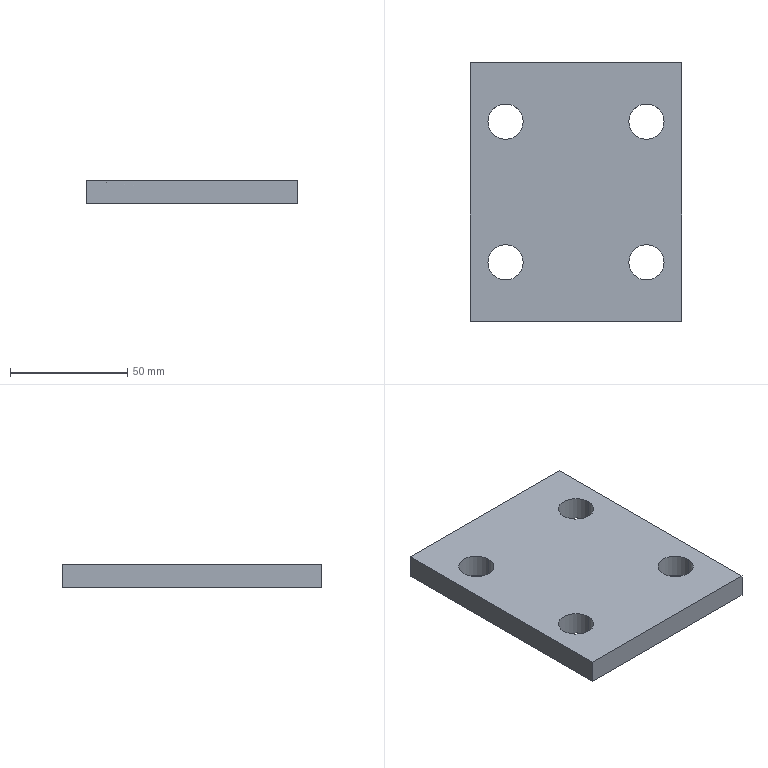Part | SolidWorks | features ICE 2, Extrusion 1 | 1 solid | 14 faces | box 90 x 110 x 10 mm | volume 91931 mm3 | cylinder 8 | plane 6 | commonest cylinder face diameters 15 x8
STEP:
#1=CARTESIAN_POINT('',(72.5,30.,0.));
#2=VERTEX_POINT('',#1);
#3=CARTESIAN_POINT('',(87.5,30.,0.));
#4=VERTEX_POINT('',#3);
#5=CARTESIAN_POINT('',(80.,30.,0.));
#6=DIRECTION('',(0.,0.,1.));
#7=DIRECTION('',(1.,0.,0.));
#8=AXIS2_PLACEMENT_3D('',#5,#6,#7);
#9=CIRCLE('',#8,7.5);
#10=EDGE_CURVE('',#2,#4,#9,.T.);
#11=ORIENTED_EDGE('',*,*,#10,.F.);
#12=CARTESIAN_POINT('',(72.5,30.,10.));
#13=VERTEX_POINT('',#12);
#14=CARTESIAN_POINT('',(72.5,30.,0.));
#15=DIRECTION('',(0.,0.,1.));
#16=VECTOR('',#15,1000.);
#17=LINE('',#14,#16);
#18=EDGE_CURVE('',#2,#13,#17,.T.);
#19=ORIENTED_EDGE('',*,*,#18,.T.);
#20=CARTESIAN_POINT('',(87.5,30.,10.));
#21=VERTEX_POINT('',#20);
#22=CARTESIAN_POINT('',(80.,30.,10.));
#23=DIRECTION('',(0.,0.,1.));
#24=DIRECTION('',(1.,0.,0.));
#25=AXIS2_PLACEMENT_3D('',#22,#23,#24);
#26=CIRCLE('',#25,7.5);
#27=EDGE_CURVE('',#13,#21,#26,.T.);
#28=ORIENTED_EDGE('',*,*,#27,.T.);
#29=CARTESIAN_POINT('',(87.5,30.,0.));
#30=DIRECTION('',(0.,0.,1.));
#31=VECTOR('',#30,1000.);
#32=LINE('',#29,#31);
#33=EDGE_CURVE('',#4,#21,#32,.T.);
#34=ORIENTED_EDGE('',*,*,#33,.F.);
#35=EDGE_LOOP('',(#11,#19,#28,#34));
#36=FACE_OUTER_BOUND('',#35,.T.);
#37=CARTESIAN_POINT('',(80.,30.,0.));
#38=DIRECTION('',(0.,0.,1.));
#39=DIRECTION('',(1.,0.,0.));
#40=AXIS2_PLACEMENT_3D('',#37,#38,#39);
#41=CYLINDRICAL_SURFACE('',#40,7.5);
#42=ADVANCED_FACE('',(#36),#41,.F.);
#43=CARTESIAN_POINT('',(12.5,30.,0.));
#44=VERTEX_POINT('',#43);
#45=CARTESIAN_POINT('',(27.5,30.,0.));
#46=VERTEX_POINT('',#45);
#47=CARTESIAN_POINT('',(20.,30.,0.));
#48=DIRECTION('',(0.,0.,1.));
#49=DIRECTION('',(1.,0.,0.));
#50=AXIS2_PLACEMENT_3D('',#47,#48,#49);
#51=CIRCLE('',#50,7.5);
#52=EDGE_CURVE('',#44,#46,#51,.T.);
#53=ORIENTED_EDGE('',*,*,#52,.F.);
#54=CARTESIAN_POINT('',(12.5,30.,10.));
#55=VERTEX_POINT('',#54);
#56=CARTESIAN_POINT('',(12.5,30.,0.));
#57=DIRECTION('',(0.,0.,1.));
#58=VECTOR('',#57,1000.);
#59=LINE('',#56,#58);
#60=EDGE_CURVE('',#44,#55,#59,.T.);
#61=ORIENTED_EDGE('',*,*,#60,.T.);
#62=CARTESIAN_POINT('',(27.5,30.,10.));
#63=VERTEX_POINT('',#62);
#64=CARTESIAN_POINT('',(20.,30.,10.));
#65=DIRECTION('',(0.,0.,1.));
#66=DIRECTION('',(1.,0.,0.));
#67=AXIS2_PLACEMENT_3D('',#64,#65,#66);
#68=CIRCLE('',#67,7.5);
#69=EDGE_CURVE('',#55,#63,#68,.T.);
#70=ORIENTED_EDGE('',*,*,#69,.T.);
#71=CARTESIAN_POINT('',(27.5,30.,0.));
#72=DIRECTION('',(0.,0.,1.));
#73=VECTOR('',#72,1000.);
#74=LINE('',#71,#73);
#75=EDGE_CURVE('',#46,#63,#74,.T.);
#76=ORIENTED_EDGE('',*,*,#75,.F.);
#77=EDGE_LOOP('',(#53,#61,#70,#76));
#78=FACE_OUTER_BOUND('',#77,.T.);
#79=CARTESIAN_POINT('',(20.,30.,0.));
#80=DIRECTION('',(0.,0.,1.));
#81=DIRECTION('',(1.,0.,0.));
#82=AXIS2_PLACEMENT_3D('',#79,#80,#81);
#83=CYLINDRICAL_SURFACE('',#82,7.5);
#84=ADVANCED_FACE('',(#78),#83,.F.);
#85=CARTESIAN_POINT('',(12.5,90.,0.));
#86=VERTEX_POINT('',#85);
#87=CARTESIAN_POINT('',(27.5,90.,0.));
#88=VERTEX_POINT('',#87);
#89=CARTESIAN_POINT('',(20.,90.,0.));
#90=DIRECTION('',(0.,0.,1.));
#91=DIRECTION('',(1.,0.,0.));
#92=AXIS2_PLACEMENT_3D('',#89,#90,#91);
#93=CIRCLE('',#92,7.5);
#94=EDGE_CURVE('',#86,#88,#93,.T.);
#95=ORIENTED_EDGE('',*,*,#94,.F.);
#96=CARTESIAN_POINT('',(12.5,90.,10.));
#97=VERTEX_POINT('',#96);
#98=CARTESIAN_POINT('',(12.5,90.,0.));
#99=DIRECTION('',(0.,0.,1.));
#100=VECTOR('',#99,1000.);
#101=LINE('',#98,#100);
#102=EDGE_CURVE('',#86,#97,#101,.T.);
#103=ORIENTED_EDGE('',*,*,#102,.T.);
#104=CARTESIAN_POINT('',(27.5,90.,10.));
#105=VERTEX_POINT('',#104);
#106=CARTESIAN_POINT('',(20.,90.,10.));
#107=DIRECTION('',(0.,0.,1.));
#108=DIRECTION('',(1.,0.,0.));
#109=AXIS2_PLACEMENT_3D('',#106,#107,#108);
#110=CIRCLE('',#109,7.5);
#111=EDGE_CURVE('',#97,#105,#110,.T.);
#112=ORIENTED_EDGE('',*,*,#111,.T.);
#113=CARTESIAN_POINT('',(27.5,90.,0.));
#114=DIRECTION('',(0.,0.,1.));
#115=VECTOR('',#114,1000.);
#116=LINE('',#113,#115);
#117=EDGE_CURVE('',#88,#105,#116,.T.);
#118=ORIENTED_EDGE('',*,*,#117,.F.);
#119=EDGE_LOOP('',(#95,#103,#112,#118));
#120=FACE_OUTER_BOUND('',#119,.T.);
#121=CARTESIAN_POINT('',(20.,90.,0.));
#122=DIRECTION('',(0.,0.,1.));
#123=DIRECTION('',(1.,0.,0.));
#124=AXIS2_PLACEMENT_3D('',#121,#122,#123);
#125=CYLINDRICAL_SURFACE('',#124,7.5);
#126=ADVANCED_FACE('',(#120),#125,.F.);
#127=CARTESIAN_POINT('',(72.5,90.,0.));
#128=VERTEX_POINT('',#127);
#129=CARTESIAN_POINT('',(87.5,90.,0.));
#130=VERTEX_POINT('',#129);
#131=CARTESIAN_POINT('',(80.,90.,0.));
#132=DIRECTION('',(0.,0.,1.));
#133=DIRECTION('',(1.,0.,0.));
#134=AXIS2_PLACEMENT_3D('',#131,#132,#133);
#135=CIRCLE('',#134,7.5);
#136=EDGE_CURVE('',#128,#130,#135,.T.);
#137=ORIENTED_EDGE('',*,*,#136,.F.);
#138=CARTESIAN_POINT('',(72.5,90.,10.));
#139=VERTEX_POINT('',#138);
#140=CARTESIAN_POINT('',(72.5,90.,0.));
#141=DIRECTION('',(0.,0.,1.));
#142=VECTOR('',#141,1000.);
#143=LINE('',#140,#142);
#144=EDGE_CURVE('',#128,#139,#143,.T.);
#145=ORIENTED_EDGE('',*,*,#144,.T.);
#146=CARTESIAN_POINT('',(87.5,90.,10.));
#147=VERTEX_POINT('',#146);
#148=CARTESIAN_POINT('',(80.,90.,10.));
#149=DIRECTION('',(0.,0.,1.));
#150=DIRECTION('',(1.,0.,0.));
#151=AXIS2_PLACEMENT_3D('',#148,#149,#150);
#152=CIRCLE('',#151,7.5);
#153=EDGE_CURVE('',#139,#147,#152,.T.);
#154=ORIENTED_EDGE('',*,*,#153,.T.);
#155=CARTESIAN_POINT('',(87.5,90.,0.));
#156=DIRECTION('',(0.,0.,1.));
#157=VECTOR('',#156,1000.);
#158=LINE('',#155,#157);
#159=EDGE_CURVE('',#130,#147,#158,.T.);
#160=ORIENTED_EDGE('',*,*,#159,.F.);
#161=EDGE_LOOP('',(#137,#145,#154,#160));
#162=FACE_OUTER_BOUND('',#161,.T.);
#163=CARTESIAN_POINT('',(80.,90.,0.));
#164=DIRECTION('',(0.,0.,1.));
#165=DIRECTION('',(1.,0.,0.));
#166=AXIS2_PLACEMENT_3D('',#163,#164,#165);
#167=CYLINDRICAL_SURFACE('',#166,7.5);
#168=ADVANCED_FACE('',(#162),#167,.F.);
#169=CARTESIAN_POINT('',(80.,90.,10.));
#170=DIRECTION('',(0.,0.,1.));
#171=DIRECTION('',(1.,0.,0.));
#172=AXIS2_PLACEMENT_3D('',#169,#170,#171);
#173=CIRCLE('',#172,7.5);
#174=EDGE_CURVE('',#147,#139,#173,.T.);
#175=ORIENTED_EDGE('',*,*,#174,.F.);
#176=ORIENTED_EDGE('',*,*,#153,.F.);
#177=EDGE_LOOP('',(#175,#176));
#178=FACE_BOUND('',#177,.T.);
#179=CARTESIAN_POINT('',(20.,90.,10.));
#180=DIRECTION('',(0.,0.,1.));
#181=DIRECTION('',(1.,0.,0.));
#182=AXIS2_PLACEMENT_3D('',#179,#180,#181);
#183=CIRCLE('',#182,7.5);
#184=EDGE_CURVE('',#105,#97,#183,.T.);
#185=ORIENTED_EDGE('',*,*,#184,.F.);
#186=ORIENTED_EDGE('',*,*,#111,.F.);
#187=EDGE_LOOP('',(#185,#186));
#188=FACE_BOUND('',#187,.T.);
#189=CARTESIAN_POINT('',(20.,30.,10.));
#190=DIRECTION('',(0.,0.,1.));
#191=DIRECTION('',(1.,0.,0.));
#192=AXIS2_PLACEMENT_3D('',#189,#190,#191);
#193=CIRCLE('',#192,7.5);
#194=EDGE_CURVE('',#63,#55,#193,.T.);
#195=ORIENTED_EDGE('',*,*,#194,.F.);
#196=ORIENTED_EDGE('',*,*,#69,.F.);
#197=EDGE_LOOP('',(#195,#196));
#198=FACE_BOUND('',#197,.T.);
#199=CARTESIAN_POINT('',(80.,30.,10.));
#200=DIRECTION('',(0.,0.,1.));
#201=DIRECTION('',(1.,0.,0.));
#202=AXIS2_PLACEMENT_3D('',#199,#200,#201);
#203=CIRCLE('',#202,7.5);
#204=EDGE_CURVE('',#21,#13,#203,.T.);
#205=ORIENTED_EDGE('',*,*,#204,.F.);
#206=ORIENTED_EDGE('',*,*,#27,.F.);
#207=EDGE_LOOP('',(#205,#206));
#208=FACE_BOUND('',#207,.T.);
#209=CARTESIAN_POINT('',(95.,5.,10.));
#210=VERTEX_POINT('',#209);
#211=CARTESIAN_POINT('',(95.,115.,10.));
#212=VERTEX_POINT('',#211);
#213=CARTESIAN_POINT('',(95.,60.,10.));
#214=DIRECTION('',(0.,1.,0.));
#215=VECTOR('',#214,1000.);
#216=LINE('',#213,#215);
#217=EDGE_CURVE('',#210,#212,#216,.T.);
#218=ORIENTED_EDGE('',*,*,#217,.T.);
#219=CARTESIAN_POINT('',(5.,115.,10.));
#220=VERTEX_POINT('',#219);
#221=CARTESIAN_POINT('',(95.,115.,10.));
#222=DIRECTION('',(-1.,0.,0.));
#223=VECTOR('',#222,1000.);
#224=LINE('',#221,#223);
#225=EDGE_CURVE('',#212,#220,#224,.T.);
#226=ORIENTED_EDGE('',*,*,#225,.T.);
#227=CARTESIAN_POINT('',(5.,5.,10.));
#228=VERTEX_POINT('',#227);
#229=CARTESIAN_POINT('',(5.,115.,10.));
#230=DIRECTION('',(0.,-1.,0.));
#231=VECTOR('',#230,1000.);
#232=LINE('',#229,#231);
#233=EDGE_CURVE('',#220,#228,#232,.T.);
#234=ORIENTED_EDGE('',*,*,#233,.T.);
#235=CARTESIAN_POINT('',(5.,5.,10.));
#236=DIRECTION('',(1.,0.,0.));
#237=VECTOR('',#236,1000.);
#238=LINE('',#235,#237);
#239=EDGE_CURVE('',#228,#210,#238,.T.);
#240=ORIENTED_EDGE('',*,*,#239,.T.);
#241=EDGE_LOOP('',(#218,#226,#234,#240));
#242=FACE_OUTER_BOUND('',#241,.T.);
#243=CARTESIAN_POINT('',(0.,0.,10.));
#244=DIRECTION('',(0.,0.,-1.));
#245=DIRECTION('',(-1.,0.,0.));
#246=AXIS2_PLACEMENT_3D('',#243,#244,#245);
#247=PLANE('',#246);
#248=ADVANCED_FACE('',(#178,#188,#198,#208,#242),#247,.F.);
#249=CARTESIAN_POINT('',(80.,90.,0.));
#250=DIRECTION('',(0.,0.,1.));
#251=DIRECTION('',(1.,0.,0.));
#252=AXIS2_PLACEMENT_3D('',#249,#250,#251);
#253=CIRCLE('',#252,7.5);
#254=EDGE_CURVE('',#130,#128,#253,.T.);
#255=ORIENTED_EDGE('',*,*,#254,.T.);
#256=ORIENTED_EDGE('',*,*,#136,.T.);
#257=EDGE_LOOP('',(#255,#256));
#258=FACE_BOUND('',#257,.T.);
#259=CARTESIAN_POINT('',(20.,90.,0.));
#260=DIRECTION('',(0.,0.,1.));
#261=DIRECTION('',(1.,0.,0.));
#262=AXIS2_PLACEMENT_3D('',#259,#260,#261);
#263=CIRCLE('',#262,7.5);
#264=EDGE_CURVE('',#88,#86,#263,.T.);
#265=ORIENTED_EDGE('',*,*,#264,.T.);
#266=ORIENTED_EDGE('',*,*,#94,.T.);
#267=EDGE_LOOP('',(#265,#266));
#268=FACE_BOUND('',#267,.T.);
#269=CARTESIAN_POINT('',(20.,30.,0.));
#270=DIRECTION('',(0.,0.,1.));
#271=DIRECTION('',(1.,0.,0.));
#272=AXIS2_PLACEMENT_3D('',#269,#270,#271);
#273=CIRCLE('',#272,7.5);
#274=EDGE_CURVE('',#46,#44,#273,.T.);
#275=ORIENTED_EDGE('',*,*,#274,.T.);
#276=ORIENTED_EDGE('',*,*,#52,.T.);
#277=EDGE_LOOP('',(#275,#276));
#278=FACE_BOUND('',#277,.T.);
#279=CARTESIAN_POINT('',(80.,30.,0.));
#280=DIRECTION('',(0.,0.,1.));
#281=DIRECTION('',(1.,0.,0.));
#282=AXIS2_PLACEMENT_3D('',#279,#280,#281);
#283=CIRCLE('',#282,7.5);
#284=EDGE_CURVE('',#4,#2,#283,.T.);
#285=ORIENTED_EDGE('',*,*,#284,.T.);
#286=ORIENTED_EDGE('',*,*,#10,.T.);
#287=EDGE_LOOP('',(#285,#286));
#288=FACE_BOUND('',#287,.T.);
#289=CARTESIAN_POINT('',(95.,115.,0.));
#290=VERTEX_POINT('',#289);
#291=CARTESIAN_POINT('',(5.,115.,0.));
#292=VERTEX_POINT('',#291);
#293=CARTESIAN_POINT('',(95.,115.,0.));
#294=DIRECTION('',(-1.,0.,0.));
#295=VECTOR('',#294,1000.);
#296=LINE('',#293,#295);
#297=EDGE_CURVE('',#290,#292,#296,.T.);
#298=ORIENTED_EDGE('',*,*,#297,.F.);
#299=CARTESIAN_POINT('',(95.,5.,0.));
#300=VERTEX_POINT('',#299);
#301=CARTESIAN_POINT('',(95.,60.,0.));
#302=DIRECTION('',(0.,1.,0.));
#303=VECTOR('',#302,1000.);
#304=LINE('',#301,#303);
#305=EDGE_CURVE('',#300,#290,#304,.T.);
#306=ORIENTED_EDGE('',*,*,#305,.F.);
#307=CARTESIAN_POINT('',(5.,5.,0.));
#308=VERTEX_POINT('',#307);
#309=CARTESIAN_POINT('',(5.,5.,0.));
#310=DIRECTION('',(1.,0.,0.));
#311=VECTOR('',#310,1000.);
#312=LINE('',#309,#311);
#313=EDGE_CURVE('',#308,#300,#312,.T.);
#314=ORIENTED_EDGE('',*,*,#313,.F.);
#315=CARTESIAN_POINT('',(5.,115.,0.));
#316=DIRECTION('',(0.,-1.,0.));
#317=VECTOR('',#316,1000.);
#318=LINE('',#315,#317);
#319=EDGE_CURVE('',#292,#308,#318,.T.);
#320=ORIENTED_EDGE('',*,*,#319,.F.);
#321=EDGE_LOOP('',(#298,#306,#314,#320));
#322=FACE_OUTER_BOUND('',#321,.T.);
#323=CARTESIAN_POINT('',(0.,0.,0.));
#324=DIRECTION('',(0.,0.,-1.));
#325=DIRECTION('',(-1.,0.,0.));
#326=AXIS2_PLACEMENT_3D('',#323,#324,#325);
#327=PLANE('',#326);
#328=ADVANCED_FACE('',(#258,#268,#278,#288,#322),#327,.T.);
#329=ORIENTED_EDGE('',*,*,#144,.F.);
#330=ORIENTED_EDGE('',*,*,#254,.F.);
#331=ORIENTED_EDGE('',*,*,#159,.T.);
#332=ORIENTED_EDGE('',*,*,#174,.T.);
#333=EDGE_LOOP('',(#329,#330,#331,#332));
#334=FACE_OUTER_BOUND('',#333,.T.);
#335=CARTESIAN_POINT('',(80.,90.,0.));
#336=DIRECTION('',(0.,0.,1.));
#337=DIRECTION('',(1.,0.,0.));
#338=AXIS2_PLACEMENT_3D('',#335,#336,#337);
#339=CYLINDRICAL_SURFACE('',#338,7.5);
#340=ADVANCED_FACE('',(#334),#339,.F.);
#341=ORIENTED_EDGE('',*,*,#102,.F.);
#342=ORIENTED_EDGE('',*,*,#264,.F.);
#343=ORIENTED_EDGE('',*,*,#117,.T.);
#344=ORIENTED_EDGE('',*,*,#184,.T.);
#345=EDGE_LOOP('',(#341,#342,#343,#344));
#346=FACE_OUTER_BOUND('',#345,.T.);
#347=CARTESIAN_POINT('',(20.,90.,0.));
#348=DIRECTION('',(0.,0.,1.));
#349=DIRECTION('',(1.,0.,0.));
#350=AXIS2_PLACEMENT_3D('',#347,#348,#349);
#351=CYLINDRICAL_SURFACE('',#350,7.5);
#352=ADVANCED_FACE('',(#346),#351,.F.);
#353=ORIENTED_EDGE('',*,*,#60,.F.);
#354=ORIENTED_EDGE('',*,*,#274,.F.);
#355=ORIENTED_EDGE('',*,*,#75,.T.);
#356=ORIENTED_EDGE('',*,*,#194,.T.);
#357=EDGE_LOOP('',(#353,#354,#355,#356));
#358=FACE_OUTER_BOUND('',#357,.T.);
#359=CARTESIAN_POINT('',(20.,30.,0.));
#360=DIRECTION('',(0.,0.,1.));
#361=DIRECTION('',(1.,0.,0.));
#362=AXIS2_PLACEMENT_3D('',#359,#360,#361);
#363=CYLINDRICAL_SURFACE('',#362,7.5);
#364=ADVANCED_FACE('',(#358),#363,.F.);
#365=ORIENTED_EDGE('',*,*,#18,.F.);
#366=ORIENTED_EDGE('',*,*,#284,.F.);
#367=ORIENTED_EDGE('',*,*,#33,.T.);
#368=ORIENTED_EDGE('',*,*,#204,.T.);
#369=EDGE_LOOP('',(#365,#366,#367,#368));
#370=FACE_OUTER_BOUND('',#369,.T.);
#371=CARTESIAN_POINT('',(80.,30.,0.));
#372=DIRECTION('',(0.,0.,1.));
#373=DIRECTION('',(1.,0.,0.));
#374=AXIS2_PLACEMENT_3D('',#371,#372,#373);
#375=CYLINDRICAL_SURFACE('',#374,7.5);
#376=ADVANCED_FACE('',(#370),#375,.F.);
#377=ORIENTED_EDGE('',*,*,#217,.F.);
#378=CARTESIAN_POINT('',(95.,5.,0.));
#379=DIRECTION('',(0.,0.,1.));
#380=VECTOR('',#379,1000.);
#381=LINE('',#378,#380);
#382=EDGE_CURVE('',#300,#210,#381,.T.);
#383=ORIENTED_EDGE('',*,*,#382,.F.);
#384=ORIENTED_EDGE('',*,*,#305,.T.);
#385=CARTESIAN_POINT('',(95.,115.,0.));
#386=DIRECTION('',(0.,0.,1.));
#387=VECTOR('',#386,1000.);
#388=LINE('',#385,#387);
#389=EDGE_CURVE('',#290,#212,#388,.T.);
#390=ORIENTED_EDGE('',*,*,#389,.T.);
#391=EDGE_LOOP('',(#377,#383,#384,#390));
#392=FACE_OUTER_BOUND('',#391,.T.);
#393=CARTESIAN_POINT('',(95.,60.,0.));
#394=DIRECTION('',(1.,0.,0.));
#395=DIRECTION('',(0.,0.,-1.));
#396=AXIS2_PLACEMENT_3D('',#393,#394,#395);
#397=PLANE('',#396);
#398=ADVANCED_FACE('',(#392),#397,.T.);
#399=ORIENTED_EDGE('',*,*,#239,.F.);
#400=CARTESIAN_POINT('',(5.,5.,0.));
#401=DIRECTION('',(0.,0.,1.));
#402=VECTOR('',#401,1000.);
#403=LINE('',#400,#402);
#404=EDGE_CURVE('',#308,#228,#403,.T.);
#405=ORIENTED_EDGE('',*,*,#404,.F.);
#406=ORIENTED_EDGE('',*,*,#313,.T.);
#407=ORIENTED_EDGE('',*,*,#382,.T.);
#408=EDGE_LOOP('',(#399,#405,#406,#407));
#409=FACE_OUTER_BOUND('',#408,.T.);
#410=CARTESIAN_POINT('',(5.,5.,0.));
#411=DIRECTION('',(0.,-1.,0.));
#412=DIRECTION('',(0.,0.,-1.));
#413=AXIS2_PLACEMENT_3D('',#410,#411,#412);
#414=PLANE('',#413);
#415=ADVANCED_FACE('',(#409),#414,.T.);
#416=ORIENTED_EDGE('',*,*,#233,.F.);
#417=CARTESIAN_POINT('',(5.,115.,0.));
#418=DIRECTION('',(0.,0.,1.));
#419=VECTOR('',#418,1000.);
#420=LINE('',#417,#419);
#421=EDGE_CURVE('',#292,#220,#420,.T.);
#422=ORIENTED_EDGE('',*,*,#421,.F.);
#423=ORIENTED_EDGE('',*,*,#319,.T.);
#424=ORIENTED_EDGE('',*,*,#404,.T.);
#425=EDGE_LOOP('',(#416,#422,#423,#424));
#426=FACE_OUTER_BOUND('',#425,.T.);
#427=CARTESIAN_POINT('',(5.,115.,0.));
#428=DIRECTION('',(-1.,0.,0.));
#429=DIRECTION('',(0.,0.,1.));
#430=AXIS2_PLACEMENT_3D('',#427,#428,#429);
#431=PLANE('',#430);
#432=ADVANCED_FACE('',(#426),#431,.T.);
#433=ORIENTED_EDGE('',*,*,#225,.F.);
#434=ORIENTED_EDGE('',*,*,#389,.F.);
#435=ORIENTED_EDGE('',*,*,#297,.T.);
#436=ORIENTED_EDGE('',*,*,#421,.T.);
#437=EDGE_LOOP('',(#433,#434,#435,#436));
#438=FACE_OUTER_BOUND('',#437,.T.);
#439=CARTESIAN_POINT('',(95.,115.,0.));
#440=DIRECTION('',(0.,1.,0.));
#441=DIRECTION('',(0.,0.,1.));
#442=AXIS2_PLACEMENT_3D('',#439,#440,#441);
#443=PLANE('',#442);
#444=ADVANCED_FACE('',(#438),#443,.T.);
#445=CLOSED_SHELL('',(#42,#84,#126,#168,#248,#328,#340,#352,#364,#376,#398,#415,#432,#444));
#446=MANIFOLD_SOLID_BREP('',#445);
#447=CARTESIAN_POINT('',(0.,0.,0.));
#448=DIRECTION('',(0.,0.,1.));
#449=DIRECTION('',(1.,0.,0.));
#450=AXIS2_PLACEMENT_3D('',#447,#448,#449);
#451=(LENGTH_UNIT()NAMED_UNIT(*)SI_UNIT(.MILLI.,.METRE.));
#452=UNCERTAINTY_MEASURE_WITH_UNIT(LENGTH_MEASURE(0.00001),#451,'','');
#453=(NAMED_UNIT(*)PLANE_ANGLE_UNIT()SI_UNIT($,.RADIAN.));
#454=(NAMED_UNIT(*)SI_UNIT($,.STERADIAN.)SOLID_ANGLE_UNIT());
#455=(GEOMETRIC_REPRESENTATION_CONTEXT(3)GLOBAL_UNCERTAINTY_ASSIGNED_CONTEXT((#452))GLOBAL_UNIT_ASSIGNED_CONTEXT((#451,#453,#454))REPRESENTATION_CONTEXT('',''));
#456=ADVANCED_BREP_SHAPE_REPRESENTATION('',(#446,#450),#455);